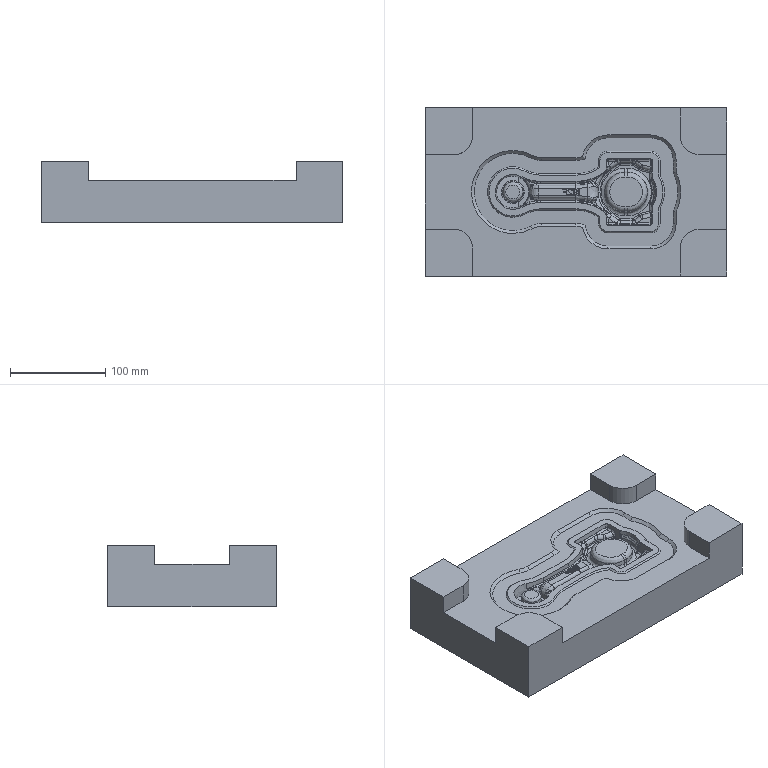Part | 1 solid | 378 faces | box 317 x 177 x 65 mm | volume 2628829 mm3 | plane 162 | spline 124 | cylinder 54 | cone 16 | torus 14 | sphere 8 | commonest cylinder face diameters 4.056 x24 8.112 x10 3.042 x6 40 x4 2.028 x2 6.084 x2